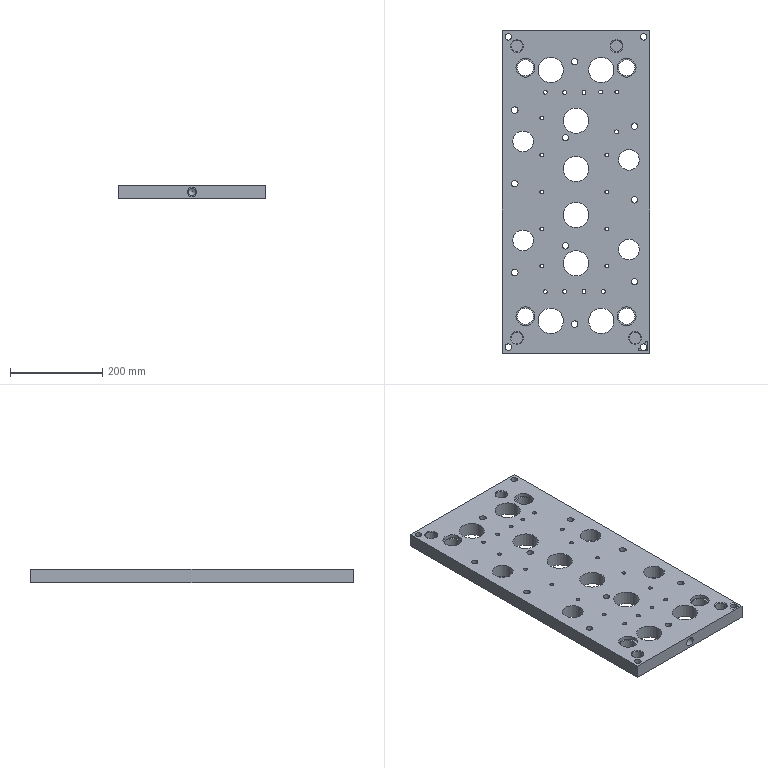Part | STEP file | DZDB | 1 solid | 184 faces | box 320 x 700 x 30 mm | volume 5578536 mm3 | cylinder 108 | plane 63 | cone 13 | commonest cylinder face diameters 14 x33 20 x23 8.5 x19 17.4 x9 55 x8 25 x4